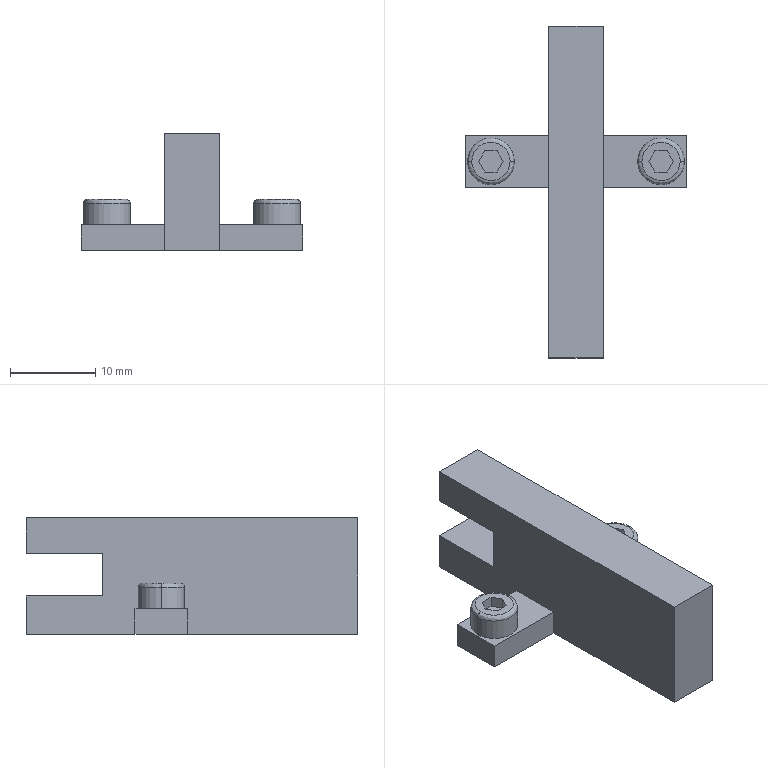Part | SolidWorks | features BaseBody 1 | 1 solid | 48 faces | box 26 x 39 x 13.7 mm | volume 3551 mm3 | plane 36 | cylinder 8 | spline 4 | commonest cylinder face diameters 3.2 x4 5.5 x4
STEP:
#1=CARTESIAN_POINT('',(-7.75,0.,6.));
#2=VERTEX_POINT('',#1);
#3=CARTESIAN_POINT('',(-12.25,0.,6.));
#4=VERTEX_POINT('',#3);
#5=CARTESIAN_POINT('',(-7.75,0.,6.));
#6=CARTESIAN_POINT('',(-7.75,-4.5,6.));
#7=CARTESIAN_POINT('',(-12.25,-4.5,6.));
#8=CARTESIAN_POINT('',(-12.25,0.,6.));
#9=(BOUNDED_CURVE()B_SPLINE_CURVE(3,(#5,#6,#7,#8),.UNSPECIFIED.,.F.,.F.)B_SPLINE_CURVE_WITH_KNOTS((4,4),(0.,1.),.UNSPECIFIED.)CURVE()GEOMETRIC_REPRESENTATION_ITEM()RATIONAL_B_SPLINE_CURVE((1.,0.3333,0.3333,1.))REPRESENTATION_ITEM(''));
#10=EDGE_CURVE('',#2,#4,#9,.T.);
#11=ORIENTED_EDGE('',*,*,#10,.T.);
#12=CARTESIAN_POINT('',(-12.75,0.,5.5));
#13=VERTEX_POINT('',#12);
#14=CARTESIAN_POINT('',(-12.25,0.,5.5));
#15=DIRECTION('',(0.,-1.,0.));
#16=DIRECTION('',(-1.,0.,0.));
#17=AXIS2_PLACEMENT_3D('',#14,#15,#16);
#18=CIRCLE('',#17,0.5);
#19=EDGE_CURVE('',#4,#13,#18,.T.);
#20=ORIENTED_EDGE('',*,*,#19,.T.);
#21=CARTESIAN_POINT('',(-7.25,0.,5.5));
#22=VERTEX_POINT('',#21);
#23=CARTESIAN_POINT('',(-10.,0.,5.5));
#24=DIRECTION('',(0.,0.,-1.));
#25=DIRECTION('',(-1.,0.,0.));
#26=AXIS2_PLACEMENT_3D('',#23,#24,#25);
#27=CIRCLE('',#26,2.75);
#28=EDGE_CURVE('',#22,#13,#27,.T.);
#29=ORIENTED_EDGE('',*,*,#28,.F.);
#30=CARTESIAN_POINT('',(-7.75,0.,5.5));
#31=DIRECTION('',(0.,1.,0.));
#32=DIRECTION('',(1.,0.,0.));
#33=AXIS2_PLACEMENT_3D('',#30,#31,#32);
#34=CIRCLE('',#33,0.5);
#35=EDGE_CURVE('',#2,#22,#34,.T.);
#36=ORIENTED_EDGE('',*,*,#35,.F.);
#37=EDGE_LOOP('',(#11,#20,#29,#36));
#38=FACE_OUTER_BOUND('',#37,.T.);
#39=CARTESIAN_POINT('',(-12.25,0.,6.));
#40=CARTESIAN_POINT('',(-12.25,-4.5,6.));
#41=CARTESIAN_POINT('',(-7.75,-4.5,6.));
#42=CARTESIAN_POINT('',(-7.75,0.,6.));
#43=CARTESIAN_POINT('',(-12.543,0.,6.));
#44=CARTESIAN_POINT('',(-12.543,-5.086,6.));
#45=CARTESIAN_POINT('',(-7.457,-5.086,6.));
#46=CARTESIAN_POINT('',(-7.457,0.,6.));
#47=CARTESIAN_POINT('',(-12.75,0.,5.793));
#48=CARTESIAN_POINT('',(-12.75,-5.5,5.793));
#49=CARTESIAN_POINT('',(-7.25,-5.5,5.793));
#50=CARTESIAN_POINT('',(-7.25,0.,5.793));
#51=CARTESIAN_POINT('',(-12.75,0.,5.5));
#52=CARTESIAN_POINT('',(-12.75,-5.5,5.5));
#53=CARTESIAN_POINT('',(-7.25,-5.5,5.5));
#54=CARTESIAN_POINT('',(-7.25,0.,5.5));
#55=(BOUNDED_SURFACE()B_SPLINE_SURFACE(3,3,((#39,#40,#41,#42),(#43,#44,#45,#46),(#47,#48,#49,#50),(#51,#52,#53,#54)),.UNSPECIFIED.,.F.,.F.,.F.)B_SPLINE_SURFACE_WITH_KNOTS((4,4),(4,4),(0.,1.),(0.,1.),.UNSPECIFIED.)GEOMETRIC_REPRESENTATION_ITEM()RATIONAL_B_SPLINE_SURFACE(((1.,0.3333,0.3333,1.),(0.8047,0.2682,0.2682,0.8047),(0.8047,0.2682,0.2682,0.8047),(1.,0.3333,0.3333,1.)))REPRESENTATION_ITEM('')SURFACE());
#56=ADVANCED_FACE('',(#38),#55,.T.);
#57=CARTESIAN_POINT('',(12.25,0.,6.));
#58=VERTEX_POINT('',#57);
#59=CARTESIAN_POINT('',(7.75,0.,6.));
#60=VERTEX_POINT('',#59);
#61=CARTESIAN_POINT('',(12.25,0.,6.));
#62=CARTESIAN_POINT('',(12.25,-4.5,6.));
#63=CARTESIAN_POINT('',(7.75,-4.5,6.));
#64=CARTESIAN_POINT('',(7.75,0.,6.));
#65=(BOUNDED_CURVE()B_SPLINE_CURVE(3,(#61,#62,#63,#64),.UNSPECIFIED.,.F.,.F.)B_SPLINE_CURVE_WITH_KNOTS((4,4),(0.,1.),.UNSPECIFIED.)CURVE()GEOMETRIC_REPRESENTATION_ITEM()RATIONAL_B_SPLINE_CURVE((1.,0.3333,0.3333,1.))REPRESENTATION_ITEM(''));
#66=EDGE_CURVE('',#58,#60,#65,.T.);
#67=ORIENTED_EDGE('',*,*,#66,.T.);
#68=CARTESIAN_POINT('',(7.25,0.,5.5));
#69=VERTEX_POINT('',#68);
#70=CARTESIAN_POINT('',(7.75,0.,5.5));
#71=DIRECTION('',(0.,-1.,0.));
#72=DIRECTION('',(-1.,0.,0.));
#73=AXIS2_PLACEMENT_3D('',#70,#71,#72);
#74=CIRCLE('',#73,0.5);
#75=EDGE_CURVE('',#60,#69,#74,.T.);
#76=ORIENTED_EDGE('',*,*,#75,.T.);
#77=CARTESIAN_POINT('',(12.75,0.,5.5));
#78=VERTEX_POINT('',#77);
#79=CARTESIAN_POINT('',(10.,0.,5.5));
#80=DIRECTION('',(0.,0.,-1.));
#81=DIRECTION('',(-1.,0.,0.));
#82=AXIS2_PLACEMENT_3D('',#79,#80,#81);
#83=CIRCLE('',#82,2.75);
#84=EDGE_CURVE('',#78,#69,#83,.T.);
#85=ORIENTED_EDGE('',*,*,#84,.F.);
#86=CARTESIAN_POINT('',(12.25,0.,5.5));
#87=DIRECTION('',(0.,1.,0.));
#88=DIRECTION('',(1.,0.,0.));
#89=AXIS2_PLACEMENT_3D('',#86,#87,#88);
#90=CIRCLE('',#89,0.5);
#91=EDGE_CURVE('',#58,#78,#90,.T.);
#92=ORIENTED_EDGE('',*,*,#91,.F.);
#93=EDGE_LOOP('',(#67,#76,#85,#92));
#94=FACE_OUTER_BOUND('',#93,.T.);
#95=CARTESIAN_POINT('',(7.75,0.,6.));
#96=CARTESIAN_POINT('',(7.75,-4.5,6.));
#97=CARTESIAN_POINT('',(12.25,-4.5,6.));
#98=CARTESIAN_POINT('',(12.25,0.,6.));
#99=CARTESIAN_POINT('',(7.457,0.,6.));
#100=CARTESIAN_POINT('',(7.457,-5.086,6.));
#101=CARTESIAN_POINT('',(12.543,-5.086,6.));
#102=CARTESIAN_POINT('',(12.543,0.,6.));
#103=CARTESIAN_POINT('',(7.25,0.,5.793));
#104=CARTESIAN_POINT('',(7.25,-5.5,5.793));
#105=CARTESIAN_POINT('',(12.75,-5.5,5.793));
#106=CARTESIAN_POINT('',(12.75,0.,5.793));
#107=CARTESIAN_POINT('',(7.25,0.,5.5));
#108=CARTESIAN_POINT('',(7.25,-5.5,5.5));
#109=CARTESIAN_POINT('',(12.75,-5.5,5.5));
#110=CARTESIAN_POINT('',(12.75,0.,5.5));
#111=(BOUNDED_SURFACE()B_SPLINE_SURFACE(3,3,((#95,#96,#97,#98),(#99,#100,#101,#102),(#103,#104,#105,#106),(#107,#108,#109,#110)),.UNSPECIFIED.,.F.,.F.,.F.)B_SPLINE_SURFACE_WITH_KNOTS((4,4),(4,4),(0.,1.),(0.,1.),.UNSPECIFIED.)GEOMETRIC_REPRESENTATION_ITEM()RATIONAL_B_SPLINE_SURFACE(((1.,0.3333,0.3333,1.),(0.8047,0.2682,0.2682,0.8047),(0.8047,0.2682,0.2682,0.8047),(1.,0.3333,0.3333,1.)))REPRESENTATION_ITEM('')SURFACE());
#112=ADVANCED_FACE('',(#94),#111,.T.);
#113=CARTESIAN_POINT('',(-8.4,0.,0.));
#114=VERTEX_POINT('',#113);
#115=CARTESIAN_POINT('',(-11.6,0.,0.));
#116=VERTEX_POINT('',#115);
#117=CARTESIAN_POINT('',(-10.,0.,0.));
#118=DIRECTION('',(0.,0.,-1.));
#119=DIRECTION('',(1.,0.,0.));
#120=AXIS2_PLACEMENT_3D('',#117,#118,#119);
#121=CIRCLE('',#120,1.6);
#122=EDGE_CURVE('',#114,#116,#121,.T.);
#123=ORIENTED_EDGE('',*,*,#122,.T.);
#124=CARTESIAN_POINT('',(-11.6,0.,3.));
#125=VERTEX_POINT('',#124);
#126=CARTESIAN_POINT('',(-11.6,0.,1.5));
#127=DIRECTION('',(0.,0.,1.));
#128=VECTOR('',#127,1000.);
#129=LINE('',#126,#128);
#130=EDGE_CURVE('',#116,#125,#129,.T.);
#131=ORIENTED_EDGE('',*,*,#130,.T.);
#132=CARTESIAN_POINT('',(-8.4,0.,3.));
#133=VERTEX_POINT('',#132);
#134=CARTESIAN_POINT('',(-10.,0.,3.));
#135=DIRECTION('',(0.,0.,-1.));
#136=DIRECTION('',(1.,0.,0.));
#137=AXIS2_PLACEMENT_3D('',#134,#135,#136);
#138=CIRCLE('',#137,1.6);
#139=EDGE_CURVE('',#133,#125,#138,.T.);
#140=ORIENTED_EDGE('',*,*,#139,.F.);
#141=CARTESIAN_POINT('',(-8.4,0.,1.5));
#142=DIRECTION('',(0.,0.,1.));
#143=VECTOR('',#142,1000.);
#144=LINE('',#141,#143);
#145=EDGE_CURVE('',#114,#133,#144,.T.);
#146=ORIENTED_EDGE('',*,*,#145,.F.);
#147=EDGE_LOOP('',(#123,#131,#140,#146));
#148=FACE_OUTER_BOUND('',#147,.T.);
#149=CARTESIAN_POINT('',(-10.,0.,1.5));
#150=DIRECTION('',(0.,0.,1.));
#151=DIRECTION('',(1.,0.,0.));
#152=AXIS2_PLACEMENT_3D('',#149,#150,#151);
#153=CYLINDRICAL_SURFACE('',#152,1.6);
#154=ADVANCED_FACE('',(#148),#153,.F.);
#155=CARTESIAN_POINT('',(11.6,0.,3.));
#156=VERTEX_POINT('',#155);
#157=CARTESIAN_POINT('',(8.4,0.,3.));
#158=VERTEX_POINT('',#157);
#159=CARTESIAN_POINT('',(10.,0.,3.));
#160=DIRECTION('',(0.,0.,-1.));
#161=DIRECTION('',(-1.,0.,0.));
#162=AXIS2_PLACEMENT_3D('',#159,#160,#161);
#163=CIRCLE('',#162,1.6);
#164=EDGE_CURVE('',#156,#158,#163,.T.);
#165=ORIENTED_EDGE('',*,*,#164,.F.);
#166=CARTESIAN_POINT('',(11.6,0.,0.));
#167=VERTEX_POINT('',#166);
#168=CARTESIAN_POINT('',(11.6,0.,3.));
#169=DIRECTION('',(0.,0.,-1.));
#170=VECTOR('',#169,1000.);
#171=LINE('',#168,#170);
#172=EDGE_CURVE('',#156,#167,#171,.T.);
#173=ORIENTED_EDGE('',*,*,#172,.T.);
#174=CARTESIAN_POINT('',(8.4,0.,0.));
#175=VERTEX_POINT('',#174);
#176=CARTESIAN_POINT('',(10.,0.,0.));
#177=DIRECTION('',(0.,0.,-1.));
#178=DIRECTION('',(-1.,0.,0.));
#179=AXIS2_PLACEMENT_3D('',#176,#177,#178);
#180=CIRCLE('',#179,1.6);
#181=EDGE_CURVE('',#167,#175,#180,.T.);
#182=ORIENTED_EDGE('',*,*,#181,.T.);
#183=CARTESIAN_POINT('',(8.4,0.,3.));
#184=DIRECTION('',(0.,0.,-1.));
#185=VECTOR('',#184,1000.);
#186=LINE('',#183,#185);
#187=EDGE_CURVE('',#158,#175,#186,.T.);
#188=ORIENTED_EDGE('',*,*,#187,.F.);
#189=EDGE_LOOP('',(#165,#173,#182,#188));
#190=FACE_OUTER_BOUND('',#189,.T.);
#191=CARTESIAN_POINT('',(10.,0.,3.));
#192=DIRECTION('',(0.,0.,-1.));
#193=DIRECTION('',(-1.,0.,0.));
#194=AXIS2_PLACEMENT_3D('',#191,#192,#193);
#195=CYLINDRICAL_SURFACE('',#194,1.6);
#196=ADVANCED_FACE('',(#190),#195,.F.);
#197=CARTESIAN_POINT('',(-10.,0.,5.5));
#198=DIRECTION('',(0.,0.,-1.));
#199=DIRECTION('',(-1.,0.,0.));
#200=AXIS2_PLACEMENT_3D('',#197,#198,#199);
#201=CIRCLE('',#200,2.75);
#202=EDGE_CURVE('',#13,#22,#201,.T.);
#203=ORIENTED_EDGE('',*,*,#202,.T.);
#204=CARTESIAN_POINT('',(-7.25,0.,3.));
#205=VERTEX_POINT('',#204);
#206=CARTESIAN_POINT('',(-7.25,0.,6.));
#207=DIRECTION('',(0.,0.,-1.));
#208=VECTOR('',#207,1000.);
#209=LINE('',#206,#208);
#210=EDGE_CURVE('',#22,#205,#209,.T.);
#211=ORIENTED_EDGE('',*,*,#210,.T.);
#212=CARTESIAN_POINT('',(-12.75,0.,3.));
#213=VERTEX_POINT('',#212);
#214=CARTESIAN_POINT('',(-10.,0.,3.));
#215=DIRECTION('',(0.,0.,-1.));
#216=DIRECTION('',(-1.,0.,0.));
#217=AXIS2_PLACEMENT_3D('',#214,#215,#216);
#218=CIRCLE('',#217,2.75);
#219=EDGE_CURVE('',#213,#205,#218,.T.);
#220=ORIENTED_EDGE('',*,*,#219,.F.);
#221=CARTESIAN_POINT('',(-12.75,0.,6.));
#222=DIRECTION('',(0.,0.,-1.));
#223=VECTOR('',#222,1000.);
#224=LINE('',#221,#223);
#225=EDGE_CURVE('',#13,#213,#224,.T.);
#226=ORIENTED_EDGE('',*,*,#225,.F.);
#227=EDGE_LOOP('',(#203,#211,#220,#226));
#228=FACE_OUTER_BOUND('',#227,.T.);
#229=CARTESIAN_POINT('',(-10.,0.,6.));
#230=DIRECTION('',(0.,0.,-1.));
#231=DIRECTION('',(-1.,0.,0.));
#232=AXIS2_PLACEMENT_3D('',#229,#230,#231);
#233=CYLINDRICAL_SURFACE('',#232,2.75);
#234=ADVANCED_FACE('',(#228),#233,.T.);
#235=CARTESIAN_POINT('',(10.,0.,5.5));
#236=DIRECTION('',(0.,0.,-1.));
#237=DIRECTION('',(-1.,0.,0.));
#238=AXIS2_PLACEMENT_3D('',#235,#236,#237);
#239=CIRCLE('',#238,2.75);
#240=EDGE_CURVE('',#69,#78,#239,.T.);
#241=ORIENTED_EDGE('',*,*,#240,.T.);
#242=CARTESIAN_POINT('',(12.75,0.,3.));
#243=VERTEX_POINT('',#242);
#244=CARTESIAN_POINT('',(12.75,0.,6.));
#245=DIRECTION('',(0.,0.,-1.));
#246=VECTOR('',#245,1000.);
#247=LINE('',#244,#246);
#248=EDGE_CURVE('',#78,#243,#247,.T.);
#249=ORIENTED_EDGE('',*,*,#248,.T.);
#250=CARTESIAN_POINT('',(7.25,0.,3.));
#251=VERTEX_POINT('',#250);
#252=CARTESIAN_POINT('',(10.,0.,3.));
#253=DIRECTION('',(0.,0.,-1.));
#254=DIRECTION('',(-1.,0.,0.));
#255=AXIS2_PLACEMENT_3D('',#252,#253,#254);
#256=CIRCLE('',#255,2.75);
#257=EDGE_CURVE('',#251,#243,#256,.T.);
#258=ORIENTED_EDGE('',*,*,#257,.F.);
#259=CARTESIAN_POINT('',(7.25,0.,6.));
#260=DIRECTION('',(0.,0.,-1.));
#261=VECTOR('',#260,1000.);
#262=LINE('',#259,#261);
#263=EDGE_CURVE('',#69,#251,#262,.T.);
#264=ORIENTED_EDGE('',*,*,#263,.F.);
#265=EDGE_LOOP('',(#241,#249,#258,#264));
#266=FACE_OUTER_BOUND('',#265,.T.);
#267=CARTESIAN_POINT('',(10.,0.,6.));
#268=DIRECTION('',(0.,0.,-1.));
#269=DIRECTION('',(-1.,0.,0.));
#270=AXIS2_PLACEMENT_3D('',#267,#268,#269);
#271=CYLINDRICAL_SURFACE('',#270,2.75);
#272=ADVANCED_FACE('',(#266),#271,.T.);
#273=CARTESIAN_POINT('',(-3.175,-23.1,13.7));
#274=VERTEX_POINT('',#273);
#275=CARTESIAN_POINT('',(-3.175,15.9,13.7));
#276=VERTEX_POINT('',#275);
#277=CARTESIAN_POINT('',(-3.175,-23.1,13.7));
#278=DIRECTION('',(0.,1.,0.));
#279=VECTOR('',#278,1000.);
#280=LINE('',#277,#279);
#281=EDGE_CURVE('',#274,#276,#280,.T.);
#282=ORIENTED_EDGE('',*,*,#281,.T.);
#283=CARTESIAN_POINT('',(-3.175,15.9,9.5));
#284=VERTEX_POINT('',#283);
#285=CARTESIAN_POINT('',(-3.175,15.9,0.));
#286=DIRECTION('',(0.,0.,-1.));
#287=VECTOR('',#286,1000.);
#288=LINE('',#285,#287);
#289=EDGE_CURVE('',#276,#284,#288,.T.);
#290=ORIENTED_EDGE('',*,*,#289,.T.);
#291=CARTESIAN_POINT('',(-3.175,6.9,9.5));
#292=VERTEX_POINT('',#291);
#293=CARTESIAN_POINT('',(-3.175,-23.1,9.5));
#294=DIRECTION('',(0.,-1.,0.));
#295=VECTOR('',#294,1000.);
#296=LINE('',#293,#295);
#297=EDGE_CURVE('',#284,#292,#296,.T.);
#298=ORIENTED_EDGE('',*,*,#297,.T.);
#299=CARTESIAN_POINT('',(-3.175,6.9,4.5));
#300=VERTEX_POINT('',#299);
#301=CARTESIAN_POINT('',(-3.175,6.9,0.));
#302=DIRECTION('',(0.,0.,-1.));
#303=VECTOR('',#302,1000.);
#304=LINE('',#301,#303);
#305=EDGE_CURVE('',#292,#300,#304,.T.);
#306=ORIENTED_EDGE('',*,*,#305,.T.);
#307=CARTESIAN_POINT('',(-3.175,15.9,4.5));
#308=VERTEX_POINT('',#307);
#309=CARTESIAN_POINT('',(-3.175,-23.1,4.5));
#310=DIRECTION('',(0.,1.,0.));
#311=VECTOR('',#310,1000.);
#312=LINE('',#309,#311);
#313=EDGE_CURVE('',#300,#308,#312,.T.);
#314=ORIENTED_EDGE('',*,*,#313,.T.);
#315=CARTESIAN_POINT('',(-3.175,15.9,0.));
#316=VERTEX_POINT('',#315);
#317=CARTESIAN_POINT('',(-3.175,15.9,0.));
#318=DIRECTION('',(0.,0.,-1.));
#319=VECTOR('',#318,1000.);
#320=LINE('',#317,#319);
#321=EDGE_CURVE('',#308,#316,#320,.T.);
#322=ORIENTED_EDGE('',*,*,#321,.T.);
#323=CARTESIAN_POINT('',(-3.175,3.1,0.));
#324=VERTEX_POINT('',#323);
#325=CARTESIAN_POINT('',(-3.175,-23.1,0.));
#326=DIRECTION('',(0.,-1.,0.));
#327=VECTOR('',#326,1000.);
#328=LINE('',#325,#327);
#329=EDGE_CURVE('',#316,#324,#328,.T.);
#330=ORIENTED_EDGE('',*,*,#329,.T.);
#331=CARTESIAN_POINT('',(-3.175,3.1,3.));
#332=VERTEX_POINT('',#331);
#333=CARTESIAN_POINT('',(-3.175,3.1,0.));
#334=DIRECTION('',(0.,0.,1.));
#335=VECTOR('',#334,1000.);
#336=LINE('',#333,#335);
#337=EDGE_CURVE('',#324,#332,#336,.T.);
#338=ORIENTED_EDGE('',*,*,#337,.T.);
#339=CARTESIAN_POINT('',(-3.175,-3.1,3.));
#340=VERTEX_POINT('',#339);
#341=CARTESIAN_POINT('',(-3.175,-23.1,3.));
#342=DIRECTION('',(0.,-1.,0.));
#343=VECTOR('',#342,1000.);
#344=LINE('',#341,#343);
#345=EDGE_CURVE('',#332,#340,#344,.T.);
#346=ORIENTED_EDGE('',*,*,#345,.T.);
#347=CARTESIAN_POINT('',(-3.175,-3.1,0.));
#348=VERTEX_POINT('',#347);
#349=CARTESIAN_POINT('',(-3.175,-3.1,0.));
#350=DIRECTION('',(0.,0.,-1.));
#351=VECTOR('',#350,1000.);
#352=LINE('',#349,#351);
#353=EDGE_CURVE('',#340,#348,#352,.T.);
#354=ORIENTED_EDGE('',*,*,#353,.T.);
#355=CARTESIAN_POINT('',(-3.175,-23.1,0.));
#356=VERTEX_POINT('',#355);
#357=CARTESIAN_POINT('',(-3.175,-23.1,0.));
#358=DIRECTION('',(0.,-1.,0.));
#359=VECTOR('',#358,1000.);
#360=LINE('',#357,#359);
#361=EDGE_CURVE('',#348,#356,#360,.T.);
#362=ORIENTED_EDGE('',*,*,#361,.T.);
#363=CARTESIAN_POINT('',(-3.175,-23.1,0.));
#364=DIRECTION('',(0.,0.,1.));
#365=VECTOR('',#364,1000.);
#366=LINE('',#363,#365);
#367=EDGE_CURVE('',#356,#274,#366,.T.);
#368=ORIENTED_EDGE('',*,*,#367,.T.);
#369=EDGE_LOOP('',(#282,#290,#298,#306,#314,#322,#330,#338,#346,#354,#362,#368));
#370=FACE_OUTER_BOUND('',#369,.T.);
#371=CARTESIAN_POINT('',(-3.175,-23.1,0.));
#372=DIRECTION('',(-1.,0.,0.));
#373=DIRECTION('',(0.,0.,1.));
#374=AXIS2_PLACEMENT_3D('',#371,#372,#373);
#375=PLANE('',#374);
#376=ADVANCED_FACE('',(#370),#375,.T.);
#377=CARTESIAN_POINT('',(3.175,15.9,9.5));
#378=VERTEX_POINT('',#377);
#379=CARTESIAN_POINT('',(-3.175,15.9,9.5));
#380=DIRECTION('',(-1.,0.,0.));
#381=VECTOR('',#380,1000.);
#382=LINE('',#379,#381);
#383=EDGE_CURVE('',#378,#284,#382,.T.);
#384=ORIENTED_EDGE('',*,*,#383,.T.);
#385=ORIENTED_EDGE('',*,*,#289,.F.);
#386=CARTESIAN_POINT('',(3.175,15.9,13.7));
#387=VERTEX_POINT('',#386);
#388=CARTESIAN_POINT('',(-3.175,15.9,13.7));
#389=DIRECTION('',(1.,0.,0.));
#390=VECTOR('',#389,1000.);
#391=LINE('',#388,#390);
#392=EDGE_CURVE('',#276,#387,#391,.T.);
#393=ORIENTED_EDGE('',*,*,#392,.T.);
#394=CARTESIAN_POINT('',(3.175,15.9,0.));
#395=DIRECTION('',(0.,0.,-1.));
#396=VECTOR('',#395,1000.);
#397=LINE('',#394,#396);
#398=EDGE_CURVE('',#387,#378,#397,.T.);
#399=ORIENTED_EDGE('',*,*,#398,.T.);
#400=EDGE_LOOP('',(#384,#385,#393,#399));
#401=FACE_OUTER_BOUND('',#400,.T.);
#402=CARTESIAN_POINT('',(-3.175,15.9,0.));
#403=DIRECTION('',(0.,1.,0.));
#404=DIRECTION('',(0.,0.,1.));
#405=AXIS2_PLACEMENT_3D('',#402,#403,#404);
#406=PLANE('',#405);
#407=ADVANCED_FACE('',(#401),#406,.T.);
#408=ORIENTED_EDGE('',*,*,#281,.F.);
#409=CARTESIAN_POINT('',(3.175,-23.1,13.7));
#410=VERTEX_POINT('',#409);
#411=CARTESIAN_POINT('',(0.,-23.1,13.7));
#412=DIRECTION('',(1.,0.,0.));
#413=VECTOR('',#412,1000.);
#414=LINE('',#411,#413);
#415=EDGE_CURVE('',#274,#410,#414,.T.);
#416=ORIENTED_EDGE('',*,*,#415,.T.);
#417=CARTESIAN_POINT('',(3.175,-3.6,13.7));
#418=DIRECTION('',(0.,1.,0.));
#419=VECTOR('',#418,1000.);
#420=LINE('',#417,#419);
#421=EDGE_CURVE('',#410,#387,#420,.T.);
#422=ORIENTED_EDGE('',*,*,#421,.T.);
#423=ORIENTED_EDGE('',*,*,#392,.F.);
#424=EDGE_LOOP('',(#408,#416,#422,#423));
#425=FACE_OUTER_BOUND('',#424,.T.);
#426=CARTESIAN_POINT('',(0.,-3.6,13.7));
#427=DIRECTION('',(0.,0.,1.));
#428=DIRECTION('',(1.,0.,0.));
#429=AXIS2_PLACEMENT_3D('',#426,#427,#428);
#430=PLANE('',#429);
#431=ADVANCED_FACE('',(#425),#430,.T.);
#432=ORIENTED_EDGE('',*,*,#415,.F.);
#433=ORIENTED_EDGE('',*,*,#367,.F.);
#434=CARTESIAN_POINT('',(3.175,-23.1,0.));
#435=VERTEX_POINT('',#434);
#436=CARTESIAN_POINT('',(3.175,-23.1,0.));
#437=DIRECTION('',(1.,0.,0.));
#438=VECTOR('',#437,1000.);
#439=LINE('',#436,#438);
#440=EDGE_CURVE('',#356,#435,#439,.T.);
#441=ORIENTED_EDGE('',*,*,#440,.T.);
#442=CARTESIAN_POINT('',(3.175,-23.1,0.));
#443=DIRECTION('',(0.,0.,1.));
#444=VECTOR('',#443,1000.);
#445=LINE('',#442,#444);
#446=EDGE_CURVE('',#435,#410,#445,.T.);
#447=ORIENTED_EDGE('',*,*,#446,.T.);
#448=EDGE_LOOP('',(#432,#433,#441,#447));
#449=FACE_OUTER_BOUND('',#448,.T.);
#450=CARTESIAN_POINT('',(3.175,-23.1,0.));
#451=DIRECTION('',(0.,-1.,0.));
#452=DIRECTION('',(0.,0.,-1.));
#453=AXIS2_PLACEMENT_3D('',#450,#451,#452);
#454=PLANE('',#453);
#455=ADVANCED_FACE('',(#449),#454,.T.);
#456=CARTESIAN_POINT('',(-13.,3.1,0.));
#457=VERTEX_POINT('',#456);
#458=CARTESIAN_POINT('',(0.,3.1,0.));
#459=DIRECTION('',(-1.,0.,0.));
#460=VECTOR('',#459,1000.);
#461=LINE('',#458,#460);
#462=EDGE_CURVE('',#324,#457,#461,.T.);
#463=ORIENTED_EDGE('',*,*,#462,.F.);
#464=ORIENTED_EDGE('',*,*,#329,.F.);
#465=CARTESIAN_POINT('',(3.175,15.9,0.));
#466=VERTEX_POINT('',#465);
#467=CARTESIAN_POINT('',(0.,15.9,0.));
#468=DIRECTION('',(-1.,0.,0.));
#469=VECTOR('',#468,1000.);
#470=LINE('',#467,#469);
#471=EDGE_CURVE('',#466,#316,#470,.T.);
#472=ORIENTED_EDGE('',*,*,#471,.F.);
#473=CARTESIAN_POINT('',(3.175,3.1,0.));
#474=VERTEX_POINT('',#473);
#475=CARTESIAN_POINT('',(3.175,0.,0.));
#476=DIRECTION('',(0.,1.,0.));
#477=VECTOR('',#476,1000.);
#478=LINE('',#475,#477);
#479=EDGE_CURVE('',#474,#466,#478,.T.);
#480=ORIENTED_EDGE('',*,*,#479,.F.);
#481=CARTESIAN_POINT('',(13.,3.1,0.));
#482=VERTEX_POINT('',#481);
#483=CARTESIAN_POINT('',(0.,3.1,0.));
#484=DIRECTION('',(-1.,0.,0.));
#485=VECTOR('',#484,1000.);
#486=LINE('',#483,#485);
#487=EDGE_CURVE('',#482,#474,#486,.T.);
#488=ORIENTED_EDGE('',*,*,#487,.F.);
#489=CARTESIAN_POINT('',(13.,-3.1,0.));
#490=VERTEX_POINT('',#489);
#491=CARTESIAN_POINT('',(13.,0.,0.));
#492=DIRECTION('',(0.,1.,0.));
#493=VECTOR('',#492,1000.);
#494=LINE('',#491,#493);
#495=EDGE_CURVE('',#490,#482,#494,.T.);
#496=ORIENTED_EDGE('',*,*,#495,.F.);
#497=CARTESIAN_POINT('',(3.175,-3.1,0.));
#498=VERTEX_POINT('',#497);
#499=CARTESIAN_POINT('',(0.,-3.1,0.));
#500=DIRECTION('',(1.,0.,0.));
#501=VECTOR('',#500,1000.);
#502=LINE('',#499,#501);
#503=EDGE_CURVE('',#498,#490,#502,.T.);
#504=ORIENTED_EDGE('',*,*,#503,.F.);
#505=CARTESIAN_POINT('',(3.175,0.,0.));
#506=DIRECTION('',(0.,1.,0.));
#507=VECTOR('',#506,1000.);
#508=LINE('',#505,#507);
#509=EDGE_CURVE('',#435,#498,#508,.T.);
#510=ORIENTED_EDGE('',*,*,#509,.F.);
#511=ORIENTED_EDGE('',*,*,#440,.F.);
#512=ORIENTED_EDGE('',*,*,#361,.F.);
#513=CARTESIAN_POINT('',(-13.,-3.1,0.));
#514=VERTEX_POINT('',#513);
#515=CARTESIAN_POINT('',(0.,-3.1,0.));
#516=DIRECTION('',(1.,0.,0.));
#517=VECTOR('',#516,1000.);
#518=LINE('',#515,#517);
#519=EDGE_CURVE('',#514,#348,#518,.T.);
#520=ORIENTED_EDGE('',*,*,#519,.F.);
#521=CARTESIAN_POINT('',(-13.,0.,0.));
#522=DIRECTION('',(0.,-1.,0.));
#523=VECTOR('',#522,1000.);
#524=LINE('',#521,#523);
#525=EDGE_CURVE('',#457,#514,#524,.T.);
#526=ORIENTED_EDGE('',*,*,#525,.F.);
#527=EDGE_LOOP('',(#463,#464,#472,#480,#488,#496,#504,#510,#511,#512,#520,#526));
#528=FACE_OUTER_BOUND('',#527,.T.);
#529=ORIENTED_EDGE('',*,*,#122,.F.);
#530=CARTESIAN_POINT('',(-10.,0.,0.));
#531=DIRECTION('',(0.,0.,-1.));
#532=DIRECTION('',(1.,0.,0.));
#533=AXIS2_PLACEMENT_3D('',#530,#531,#532);
#534=CIRCLE('',#533,1.6);
#535=EDGE_CURVE('',#116,#114,#534,.T.);
#536=ORIENTED_EDGE('',*,*,#535,.F.);
#537=EDGE_LOOP('',(#529,#536));
#538=FACE_BOUND('',#537,.T.);
#539=CARTESIAN_POINT('',(10.,0.,0.));
#540=DIRECTION('',(0.,0.,-1.));
#541=DIRECTION('',(-1.,0.,0.));
#542=AXIS2_PLACEMENT_3D('',#539,#540,#541);
#543=CIRCLE('',#542,1.6);
#544=EDGE_CURVE('',#175,#167,#543,.T.);
#545=ORIENTED_EDGE('',*,*,#544,.F.);
#546=ORIENTED_EDGE('',*,*,#181,.F.);
#547=EDGE_LOOP('',(#545,#546));
#548=FACE_BOUND('',#547,.T.);
#549=CARTESIAN_POINT('',(0.,0.,0.));
#550=DIRECTION('',(0.,0.,1.));
#551=DIRECTION('',(1.,0.,0.));
#552=AXIS2_PLACEMENT_3D('',#549,#550,#551);
#553=PLANE('',#552);
#554=ADVANCED_FACE('',(#528,#538,#548),#553,.F.);
#555=ORIENTED_EDGE('',*,*,#353,.F.);
#556=CARTESIAN_POINT('',(-13.,-3.1,3.));
#557=VERTEX_POINT('',#556);
#558=CARTESIAN_POINT('',(13.,-3.1,3.));
#559=DIRECTION('',(-1.,0.,0.));
#560=VECTOR('',#559,1000.);
#561=LINE('',#558,#560);
#562=EDGE_CURVE('',#340,#557,#561,.T.);
#563=ORIENTED_EDGE('',*,*,#562,.T.);
#564=CARTESIAN_POINT('',(-13.,-3.1,0.));
#565=DIRECTION('',(0.,0.,-1.));
#566=VECTOR('',#565,1000.);
#567=LINE('',#564,#566);
#568=EDGE_CURVE('',#557,#514,#567,.T.);
#569=ORIENTED_EDGE('',*,*,#568,.T.);
#570=ORIENTED_EDGE('',*,*,#519,.T.);
#571=EDGE_LOOP('',(#555,#563,#569,#570));
#572=FACE_OUTER_BOUND('',#571,.T.);
#573=CARTESIAN_POINT('',(13.,-3.1,0.));
#574=DIRECTION('',(0.,-1.,0.));
#575=DIRECTION('',(0.,0.,-1.));
#576=AXIS2_PLACEMENT_3D('',#573,#574,#575);
#577=PLANE('',#576);
#578=ADVANCED_FACE('',(#572),#577,.T.);
#579=ORIENTED_EDGE('',*,*,#219,.T.);
#580=CARTESIAN_POINT('',(-10.,0.,3.));
#581=DIRECTION('',(0.,0.,-1.));
#582=DIRECTION('',(-1.,0.,0.));
#583=AXIS2_PLACEMENT_3D('',#580,#581,#582);
#584=CIRCLE('',#583,2.75);
#585=EDGE_CURVE('',#205,#213,#584,.T.);
#586=ORIENTED_EDGE('',*,*,#585,.T.);
#587=EDGE_LOOP('',(#579,#586));
#588=FACE_BOUND('',#587,.T.);
#589=ORIENTED_EDGE('',*,*,#345,.F.);
#590=CARTESIAN_POINT('',(-13.,3.1,3.));
#591=VERTEX_POINT('',#590);
#592=CARTESIAN_POINT('',(0.,3.1,3.));
#593=DIRECTION('',(-1.,0.,0.));
#594=VECTOR('',#593,1000.);
#595=LINE('',#592,#594);
#596=EDGE_CURVE('',#332,#591,#595,.T.);
#597=ORIENTED_EDGE('',*,*,#596,.T.);
#598=CARTESIAN_POINT('',(-13.,0.,3.));
#599=DIRECTION('',(0.,-1.,0.));
#600=VECTOR('',#599,1000.);
#601=LINE('',#598,#600);
#602=EDGE_CURVE('',#591,#557,#601,.T.);
#603=ORIENTED_EDGE('',*,*,#602,.T.);
#604=ORIENTED_EDGE('',*,*,#562,.F.);
#605=EDGE_LOOP('',(#589,#597,#603,#604));
#606=FACE_OUTER_BOUND('',#605,.T.);
#607=CARTESIAN_POINT('',(0.,0.,3.));
#608=DIRECTION('',(0.,0.,1.));
#609=DIRECTION('',(1.,0.,0.));
#610=AXIS2_PLACEMENT_3D('',#607,#608,#609);
#611=PLANE('',#610);
#612=ADVANCED_FACE('',(#588,#606),#611,.T.);
#613=ORIENTED_EDGE('',*,*,#337,.F.);
#614=ORIENTED_EDGE('',*,*,#462,.T.);
#615=CARTESIAN_POINT('',(-13.,3.1,0.));
#616=DIRECTION('',(0.,0.,1.));
#617=VECTOR('',#616,1000.);
#618=LINE('',#615,#617);
#619=EDGE_CURVE('',#457,#591,#618,.T.);
#620=ORIENTED_EDGE('',*,*,#619,.T.);
#621=ORIENTED_EDGE('',*,*,#596,.F.);
#622=EDGE_LOOP('',(#613,#614,#620,#621));
#623=FACE_OUTER_BOUND('',#622,.T.);
#624=CARTESIAN_POINT('',(-13.,3.1,0.));
#625=DIRECTION('',(0.,1.,0.));
#626=DIRECTION('',(0.,0.,1.));
#627=AXIS2_PLACEMENT_3D('',#624,#625,#626);
#628=PLANE('',#627);
#629=ADVANCED_FACE('',(#623),#628,.T.);
#630=CARTESIAN_POINT('',(3.175,15.9,4.5));
#631=VERTEX_POINT('',#630);
#632=CARTESIAN_POINT('',(-3.175,15.9,4.5));
#633=DIRECTION('',(1.,0.,0.));
#634=VECTOR('',#633,1000.);
#635=LINE('',#632,#634);
#636=EDGE_CURVE('',#308,#631,#635,.T.);
#637=ORIENTED_EDGE('',*,*,#636,.T.);
#638=CARTESIAN_POINT('',(3.175,15.9,0.));
#639=DIRECTION('',(0.,0.,-1.));
#640=VECTOR('',#639,1000.);
#641=LINE('',#638,#640);
#642=EDGE_CURVE('',#631,#466,#641,.T.);
#643=ORIENTED_EDGE('',*,*,#642,.T.);
#644=ORIENTED_EDGE('',*,*,#471,.T.);
#645=ORIENTED_EDGE('',*,*,#321,.F.);
#646=EDGE_LOOP('',(#637,#643,#644,#645));
#647=FACE_OUTER_BOUND('',#646,.T.);
#648=CARTESIAN_POINT('',(-3.175,15.9,0.));
#649=DIRECTION('',(0.,1.,0.));
#650=DIRECTION('',(0.,0.,1.));
#651=AXIS2_PLACEMENT_3D('',#648,#649,#650);
#652=PLANE('',#651);
#653=ADVANCED_FACE('',(#647),#652,.T.);
#654=CARTESIAN_POINT('',(3.175,6.9,4.5));
#655=VERTEX_POINT('',#654);
#656=CARTESIAN_POINT('',(3.175,6.9,4.5));
#657=DIRECTION('',(0.,-1.,0.));
#658=VECTOR('',#657,1000.);
#659=LINE('',#656,#658);
#660=EDGE_CURVE('',#631,#655,#659,.T.);
#661=ORIENTED_EDGE('',*,*,#660,.F.);
#662=ORIENTED_EDGE('',*,*,#636,.F.);
#663=ORIENTED_EDGE('',*,*,#313,.F.);
#664=CARTESIAN_POINT('',(3.175,6.9,4.5));
#665=DIRECTION('',(-1.,0.,0.));
#666=VECTOR('',#665,1000.);
#667=LINE('',#664,#666);
#668=EDGE_CURVE('',#655,#300,#667,.T.);
#669=ORIENTED_EDGE('',*,*,#668,.F.);
#670=EDGE_LOOP('',(#661,#662,#663,#669));
#671=FACE_OUTER_BOUND('',#670,.T.);
#672=CARTESIAN_POINT('',(3.175,6.9,4.5));
#673=DIRECTION('',(0.,0.,-1.));
#674=DIRECTION('',(-1.,0.,0.));
#675=AXIS2_PLACEMENT_3D('',#672,#673,#674);
#676=PLANE('',#675);
#677=ADVANCED_FACE('',(#671),#676,.F.);
#678=CARTESIAN_POINT('',(3.175,6.9,9.5));
#679=VERTEX_POINT('',#678);
#680=CARTESIAN_POINT('',(3.175,6.9,9.5));
#681=DIRECTION('',(0.,0.,1.));
#682=VECTOR('',#681,1000.);
#683=LINE('',#680,#682);
#684=EDGE_CURVE('',#655,#679,#683,.T.);
#685=ORIENTED_EDGE('',*,*,#684,.F.);
#686=ORIENTED_EDGE('',*,*,#668,.T.);
#687=ORIENTED_EDGE('',*,*,#305,.F.);
#688=CARTESIAN_POINT('',(3.175,6.9,9.5));
#689=DIRECTION('',(-1.,0.,0.));
#690=VECTOR('',#689,1000.);
#691=LINE('',#688,#690);
#692=EDGE_CURVE('',#679,#292,#691,.T.);
#693=ORIENTED_EDGE('',*,*,#692,.F.);
#694=EDGE_LOOP('',(#685,#686,#687,#693));
#695=FACE_OUTER_BOUND('',#694,.T.);
#696=CARTESIAN_POINT('',(3.175,6.9,9.5));
#697=DIRECTION('',(0.,-1.,0.));
#698=DIRECTION('',(0.,0.,-1.));
#699=AXIS2_PLACEMENT_3D('',#696,#697,#698);
#700=PLANE('',#699);
#701=ADVANCED_FACE('',(#695),#700,.F.);
#702=CARTESIAN_POINT('',(3.175,15.9,9.5));
#703=DIRECTION('',(0.,1.,0.));
#704=VECTOR('',#703,1000.);
#705=LINE('',#702,#704);
#706=EDGE_CURVE('',#679,#378,#705,.T.);
#707=ORIENTED_EDGE('',*,*,#706,.F.);
#708=ORIENTED_EDGE('',*,*,#692,.T.);
#709=ORIENTED_EDGE('',*,*,#297,.F.);
#710=ORIENTED_EDGE('',*,*,#383,.F.);
#711=EDGE_LOOP('',(#707,#708,#709,#710));
#712=FACE_OUTER_BOUND('',#711,.T.);
#713=CARTESIAN_POINT('',(3.175,15.9,9.5));
#714=DIRECTION('',(0.,0.,1.));
#715=DIRECTION('',(1.,0.,0.));
#716=AXIS2_PLACEMENT_3D('',#713,#714,#715);
#717=PLANE('',#716);
#718=ADVANCED_FACE('',(#712),#717,.F.);
#719=CARTESIAN_POINT('',(3.175,-3.1,3.));
#720=VERTEX_POINT('',#719);
#721=CARTESIAN_POINT('',(3.175,3.1,3.));
#722=VERTEX_POINT('',#721);
#723=CARTESIAN_POINT('',(3.175,15.9,3.));
#724=DIRECTION('',(0.,1.,0.));
#725=VECTOR('',#724,1000.);
#726=LINE('',#723,#725);
#727=EDGE_CURVE('',#720,#722,#726,.T.);
#728=ORIENTED_EDGE('',*,*,#727,.T.);
#729=CARTESIAN_POINT('',(3.175,3.1,0.));
#730=DIRECTION('',(0.,0.,-1.));
#731=VECTOR('',#730,1000.);
#732=LINE('',#729,#731);
#733=EDGE_CURVE('',#722,#474,#732,.T.);
#734=ORIENTED_EDGE('',*,*,#733,.T.);
#735=ORIENTED_EDGE('',*,*,#479,.T.);
#736=ORIENTED_EDGE('',*,*,#642,.F.);
#737=ORIENTED_EDGE('',*,*,#660,.T.);
#738=ORIENTED_EDGE('',*,*,#684,.T.);
#739=ORIENTED_EDGE('',*,*,#706,.T.);
#740=ORIENTED_EDGE('',*,*,#398,.F.);
#741=ORIENTED_EDGE('',*,*,#421,.F.);
#742=ORIENTED_EDGE('',*,*,#446,.F.);
#743=ORIENTED_EDGE('',*,*,#509,.T.);
#744=CARTESIAN_POINT('',(3.175,-3.1,0.));
#745=DIRECTION('',(0.,0.,1.));
#746=VECTOR('',#745,1000.);
#747=LINE('',#744,#746);
#748=EDGE_CURVE('',#498,#720,#747,.T.);
#749=ORIENTED_EDGE('',*,*,#748,.T.);
#750=EDGE_LOOP('',(#728,#734,#735,#736,#737,#738,#739,#740,#741,#742,#743,#749));
#751=FACE_OUTER_BOUND('',#750,.T.);
#752=CARTESIAN_POINT('',(3.175,15.9,0.));
#753=DIRECTION('',(1.,0.,0.));
#754=DIRECTION('',(0.,0.,-1.));
#755=AXIS2_PLACEMENT_3D('',#752,#753,#754);
#756=PLANE('',#755);
#757=ADVANCED_FACE('',(#751),#756,.T.);
#758=ORIENTED_EDGE('',*,*,#602,.F.);
#759=ORIENTED_EDGE('',*,*,#619,.F.);
#760=ORIENTED_EDGE('',*,*,#525,.T.);
#761=ORIENTED_EDGE('',*,*,#568,.F.);
#762=EDGE_LOOP('',(#758,#759,#760,#761));
#763=FACE_OUTER_BOUND('',#762,.T.);
#764=CARTESIAN_POINT('',(-13.,-3.1,0.));
#765=DIRECTION('',(-1.,0.,0.));
#766=DIRECTION('',(0.,0.,1.));
#767=AXIS2_PLACEMENT_3D('',#764,#765,#766);
#768=PLANE('',#767);
#769=ADVANCED_FACE('',(#763),#768,.T.);
#770=ORIENTED_EDGE('',*,*,#733,.F.);
#771=CARTESIAN_POINT('',(13.,3.1,3.));
#772=VERTEX_POINT('',#771);
#773=CARTESIAN_POINT('',(-13.,3.1,3.));
#774=DIRECTION('',(1.,0.,0.));
#775=VECTOR('',#774,1000.);
#776=LINE('',#773,#775);
#777=EDGE_CURVE('',#722,#772,#776,.T.);
#778=ORIENTED_EDGE('',*,*,#777,.T.);
#779=CARTESIAN_POINT('',(13.,3.1,0.));
#780=DIRECTION('',(0.,0.,-1.));
#781=VECTOR('',#780,1000.);
#782=LINE('',#779,#781);
#783=EDGE_CURVE('',#772,#482,#782,.T.);
#784=ORIENTED_EDGE('',*,*,#783,.T.);
#785=ORIENTED_EDGE('',*,*,#487,.T.);
#786=EDGE_LOOP('',(#770,#778,#784,#785));
#787=FACE_OUTER_BOUND('',#786,.T.);
#788=CARTESIAN_POINT('',(-13.,3.1,0.));
#789=DIRECTION('',(0.,1.,0.));
#790=DIRECTION('',(0.,0.,1.));
#791=AXIS2_PLACEMENT_3D('',#788,#789,#790);
#792=PLANE('',#791);
#793=ADVANCED_FACE('',(#787),#792,.T.);
#794=CARTESIAN_POINT('',(13.,-3.1,3.));
#795=VERTEX_POINT('',#794);
#796=CARTESIAN_POINT('',(13.,3.1,3.));
#797=DIRECTION('',(0.,-1.,0.));
#798=VECTOR('',#797,1000.);
#799=LINE('',#796,#798);
#800=EDGE_CURVE('',#772,#795,#799,.T.);
#801=ORIENTED_EDGE('',*,*,#800,.T.);
#802=CARTESIAN_POINT('',(13.,-3.1,0.));
#803=DIRECTION('',(0.,0.,-1.));
#804=VECTOR('',#803,1000.);
#805=LINE('',#802,#804);
#806=EDGE_CURVE('',#795,#490,#805,.T.);
#807=ORIENTED_EDGE('',*,*,#806,.T.);
#808=ORIENTED_EDGE('',*,*,#495,.T.);
#809=ORIENTED_EDGE('',*,*,#783,.F.);
#810=EDGE_LOOP('',(#801,#807,#808,#809));
#811=FACE_OUTER_BOUND('',#810,.T.);
#812=CARTESIAN_POINT('',(13.,3.1,0.));
#813=DIRECTION('',(1.,0.,0.));
#814=DIRECTION('',(0.,0.,-1.));
#815=AXIS2_PLACEMENT_3D('',#812,#813,#814);
#816=PLANE('',#815);
#817=ADVANCED_FACE('',(#811),#816,.T.);
#818=ORIENTED_EDGE('',*,*,#748,.F.);
#819=ORIENTED_EDGE('',*,*,#503,.T.);
#820=ORIENTED_EDGE('',*,*,#806,.F.);
#821=CARTESIAN_POINT('',(13.,-3.1,3.));
#822=DIRECTION('',(-1.,0.,0.));
#823=VECTOR('',#822,1000.);
#824=LINE('',#821,#823);
#825=EDGE_CURVE('',#795,#720,#824,.T.);
#826=ORIENTED_EDGE('',*,*,#825,.T.);
#827=EDGE_LOOP('',(#818,#819,#820,#826));
#828=FACE_OUTER_BOUND('',#827,.T.);
#829=CARTESIAN_POINT('',(13.,-3.1,0.));
#830=DIRECTION('',(0.,-1.,0.));
#831=DIRECTION('',(0.,0.,-1.));
#832=AXIS2_PLACEMENT_3D('',#829,#830,#831);
#833=PLANE('',#832);
#834=ADVANCED_FACE('',(#828),#833,.T.);
#835=ORIENTED_EDGE('',*,*,#130,.F.);
#836=ORIENTED_EDGE('',*,*,#535,.T.);
#837=ORIENTED_EDGE('',*,*,#145,.T.);
#838=CARTESIAN_POINT('',(-10.,0.,3.));
#839=DIRECTION('',(0.,0.,-1.));
#840=DIRECTION('',(1.,0.,0.));
#841=AXIS2_PLACEMENT_3D('',#838,#839,#840);
#842=CIRCLE('',#841,1.6);
#843=EDGE_CURVE('',#125,#133,#842,.T.);
#844=ORIENTED_EDGE('',*,*,#843,.F.);
#845=EDGE_LOOP('',(#835,#836,#837,#844));
#846=FACE_OUTER_BOUND('',#845,.T.);
#847=CARTESIAN_POINT('',(-10.,0.,1.5));
#848=DIRECTION('',(0.,0.,1.));
#849=DIRECTION('',(1.,0.,0.));
#850=AXIS2_PLACEMENT_3D('',#847,#848,#849);
#851=CYLINDRICAL_SURFACE('',#850,1.6);
#852=ADVANCED_FACE('',(#846),#851,.F.);
#853=ORIENTED_EDGE('',*,*,#172,.F.);
#854=CARTESIAN_POINT('',(10.,0.,3.));
#855=DIRECTION('',(0.,0.,-1.));
#856=DIRECTION('',(-1.,0.,0.));
#857=AXIS2_PLACEMENT_3D('',#854,#855,#856);
#858=CIRCLE('',#857,1.6);
#859=EDGE_CURVE('',#158,#156,#858,.T.);
#860=ORIENTED_EDGE('',*,*,#859,.F.);
#861=ORIENTED_EDGE('',*,*,#187,.T.);
#862=ORIENTED_EDGE('',*,*,#544,.T.);
#863=EDGE_LOOP('',(#853,#860,#861,#862));
#864=FACE_OUTER_BOUND('',#863,.T.);
#865=CARTESIAN_POINT('',(10.,0.,3.));
#866=DIRECTION('',(0.,0.,-1.));
#867=DIRECTION('',(-1.,0.,0.));
#868=AXIS2_PLACEMENT_3D('',#865,#866,#867);
#869=CYLINDRICAL_SURFACE('',#868,1.6);
#870=ADVANCED_FACE('',(#864),#869,.F.);
#871=ORIENTED_EDGE('',*,*,#210,.F.);
#872=ORIENTED_EDGE('',*,*,#28,.T.);
#873=ORIENTED_EDGE('',*,*,#225,.T.);
#874=ORIENTED_EDGE('',*,*,#585,.F.);
#875=EDGE_LOOP('',(#871,#872,#873,#874));
#876=FACE_OUTER_BOUND('',#875,.T.);
#877=CARTESIAN_POINT('',(-10.,0.,6.));
#878=DIRECTION('',(0.,0.,-1.));
#879=DIRECTION('',(-1.,0.,0.));
#880=AXIS2_PLACEMENT_3D('',#877,#878,#879);
#881=CYLINDRICAL_SURFACE('',#880,2.75);
#882=ADVANCED_FACE('',(#876),#881,.T.);
#883=ORIENTED_EDGE('',*,*,#257,.T.);
#884=CARTESIAN_POINT('',(10.,0.,3.));
#885=DIRECTION('',(0.,0.,-1.));
#886=DIRECTION('',(-1.,0.,0.));
#887=AXIS2_PLACEMENT_3D('',#884,#885,#886);
#888=CIRCLE('',#887,2.75);
#889=EDGE_CURVE('',#243,#251,#888,.T.);
#890=ORIENTED_EDGE('',*,*,#889,.T.);
#891=EDGE_LOOP('',(#883,#890));
#892=FACE_BOUND('',#891,.T.);
#893=ORIENTED_EDGE('',*,*,#727,.F.);
#894=ORIENTED_EDGE('',*,*,#825,.F.);
#895=ORIENTED_EDGE('',*,*,#800,.F.);
#896=ORIENTED_EDGE('',*,*,#777,.F.);
#897=EDGE_LOOP('',(#893,#894,#895,#896));
#898=FACE_OUTER_BOUND('',#897,.T.);
#899=CARTESIAN_POINT('',(0.,0.,3.));
#900=DIRECTION('',(0.,0.,1.));
#901=DIRECTION('',(1.,0.,0.));
#902=AXIS2_PLACEMENT_3D('',#899,#900,#901);
#903=PLANE('',#902);
#904=ADVANCED_FACE('',(#892,#898),#903,.T.);
#905=ORIENTED_EDGE('',*,*,#139,.T.);
#906=ORIENTED_EDGE('',*,*,#843,.T.);
#907=EDGE_LOOP('',(#905,#906));
#908=FACE_OUTER_BOUND('',#907,.T.);
#909=CARTESIAN_POINT('',(-10.,0.,3.));
#910=DIRECTION('',(0.,0.,1.));
#911=DIRECTION('',(1.,0.,0.));
#912=AXIS2_PLACEMENT_3D('',#909,#910,#911);
#913=PLANE('',#912);
#914=ADVANCED_FACE('',(#908),#913,.F.);
#915=ORIENTED_EDGE('',*,*,#859,.T.);
#916=ORIENTED_EDGE('',*,*,#164,.T.);
#917=EDGE_LOOP('',(#915,#916));
#918=FACE_OUTER_BOUND('',#917,.T.);
#919=CARTESIAN_POINT('',(10.,0.,3.));
#920=DIRECTION('',(0.,0.,1.));
#921=DIRECTION('',(1.,0.,0.));
#922=AXIS2_PLACEMENT_3D('',#919,#920,#921);
#923=PLANE('',#922);
#924=ADVANCED_FACE('',(#918),#923,.F.);
#925=ORIENTED_EDGE('',*,*,#19,.F.);
#926=CARTESIAN_POINT('',(-12.25,0.,6.));
#927=CARTESIAN_POINT('',(-12.25,4.5,6.));
#928=CARTESIAN_POINT('',(-7.75,4.5,6.));
#929=CARTESIAN_POINT('',(-7.75,0.,6.));
#930=(BOUNDED_CURVE()B_SPLINE_CURVE(3,(#926,#927,#928,#929),.UNSPECIFIED.,.F.,.F.)B_SPLINE_CURVE_WITH_KNOTS((4,4),(0.,1.),.UNSPECIFIED.)CURVE()GEOMETRIC_REPRESENTATION_ITEM()RATIONAL_B_SPLINE_CURVE((1.,0.3333,0.3333,1.))REPRESENTATION_ITEM(''));
#931=EDGE_CURVE('',#4,#2,#930,.T.);
#932=ORIENTED_EDGE('',*,*,#931,.T.);
#933=ORIENTED_EDGE('',*,*,#35,.T.);
#934=ORIENTED_EDGE('',*,*,#202,.F.);
#935=EDGE_LOOP('',(#925,#932,#933,#934));
#936=FACE_OUTER_BOUND('',#935,.T.);
#937=CARTESIAN_POINT('',(-7.75,0.,6.));
#938=CARTESIAN_POINT('',(-7.75,4.5,6.));
#939=CARTESIAN_POINT('',(-12.25,4.5,6.));
#940=CARTESIAN_POINT('',(-12.25,0.,6.));
#941=CARTESIAN_POINT('',(-7.457,0.,6.));
#942=CARTESIAN_POINT('',(-7.457,5.086,6.));
#943=CARTESIAN_POINT('',(-12.543,5.086,6.));
#944=CARTESIAN_POINT('',(-12.543,0.,6.));
#945=CARTESIAN_POINT('',(-7.25,0.,5.793));
#946=CARTESIAN_POINT('',(-7.25,5.5,5.793));
#947=CARTESIAN_POINT('',(-12.75,5.5,5.793));
#948=CARTESIAN_POINT('',(-12.75,0.,5.793));
#949=CARTESIAN_POINT('',(-7.25,0.,5.5));
#950=CARTESIAN_POINT('',(-7.25,5.5,5.5));
#951=CARTESIAN_POINT('',(-12.75,5.5,5.5));
#952=CARTESIAN_POINT('',(-12.75,0.,5.5));
#953=(BOUNDED_SURFACE()B_SPLINE_SURFACE(3,3,((#937,#938,#939,#940),(#941,#942,#943,#944),(#945,#946,#947,#948),(#949,#950,#951,#952)),.UNSPECIFIED.,.F.,.F.,.F.)B_SPLINE_SURFACE_WITH_KNOTS((4,4),(4,4),(0.,1.),(0.,1.),.UNSPECIFIED.)GEOMETRIC_REPRESENTATION_ITEM()RATIONAL_B_SPLINE_SURFACE(((1.,0.3333,0.3333,1.),(0.8047,0.2682,0.2682,0.8047),(0.8047,0.2682,0.2682,0.8047),(1.,0.3333,0.3333,1.)))REPRESENTATION_ITEM('')SURFACE());
#954=ADVANCED_FACE('',(#936),#953,.T.);
#955=ORIENTED_EDGE('',*,*,#248,.F.);
#956=ORIENTED_EDGE('',*,*,#84,.T.);
#957=ORIENTED_EDGE('',*,*,#263,.T.);
#958=ORIENTED_EDGE('',*,*,#889,.F.);
#959=EDGE_LOOP('',(#955,#956,#957,#958));
#960=FACE_OUTER_BOUND('',#959,.T.);
#961=CARTESIAN_POINT('',(10.,0.,6.));
#962=DIRECTION('',(0.,0.,-1.));
#963=DIRECTION('',(-1.,0.,0.));
#964=AXIS2_PLACEMENT_3D('',#961,#962,#963);
#965=CYLINDRICAL_SURFACE('',#964,2.75);
#966=ADVANCED_FACE('',(#960),#965,.T.);
#967=CARTESIAN_POINT('',(-10.722,1.25,6.));
#968=VERTEX_POINT('',#967);
#969=CARTESIAN_POINT('',(-9.278,1.25,6.));
#970=VERTEX_POINT('',#969);
#971=CARTESIAN_POINT('',(-10.,1.25,6.));
#972=DIRECTION('',(1.,0.,0.));
#973=VECTOR('',#972,1000.);
#974=LINE('',#971,#973);
#975=EDGE_CURVE('',#968,#970,#974,.T.);
#976=ORIENTED_EDGE('',*,*,#975,.T.);
#977=CARTESIAN_POINT('',(-8.557,0.,6.));
#978=VERTEX_POINT('',#977);
#979=CARTESIAN_POINT('',(-9.278,1.25,6.));
#980=DIRECTION('',(0.5,-0.866,0.));
#981=VECTOR('',#980,1000.);
#982=LINE('',#979,#981);
#983=EDGE_CURVE('',#970,#978,#982,.T.);
#984=ORIENTED_EDGE('',*,*,#983,.T.);
#985=CARTESIAN_POINT('',(-9.278,-1.25,6.));
#986=VERTEX_POINT('',#985);
#987=CARTESIAN_POINT('',(-8.557,0.,6.));
#988=DIRECTION('',(-0.5,-0.866,0.));
#989=VECTOR('',#988,1000.);
#990=LINE('',#987,#989);
#991=EDGE_CURVE('',#978,#986,#990,.T.);
#992=ORIENTED_EDGE('',*,*,#991,.T.);
#993=CARTESIAN_POINT('',(-10.722,-1.25,6.));
#994=VERTEX_POINT('',#993);
#995=CARTESIAN_POINT('',(-10.,-1.25,6.));
#996=DIRECTION('',(-1.,0.,0.));
#997=VECTOR('',#996,1000.);
#998=LINE('',#995,#997);
#999=EDGE_CURVE('',#986,#994,#998,.T.);
#1000=ORIENTED_EDGE('',*,*,#999,.T.);
#1001=CARTESIAN_POINT('',(-11.443,0.,6.));
#1002=VERTEX_POINT('',#1001);
#1003=CARTESIAN_POINT('',(-10.722,-1.25,6.));
#1004=DIRECTION('',(-0.5,0.866,0.));
#1005=VECTOR('',#1004,1000.);
#1006=LINE('',#1003,#1005);
#1007=EDGE_CURVE('',#994,#1002,#1006,.T.);
#1008=ORIENTED_EDGE('',*,*,#1007,.T.);
#1009=CARTESIAN_POINT('',(-11.443,0.,6.));
#1010=DIRECTION('',(0.5,0.866,0.));
#1011=VECTOR('',#1010,1000.);
#1012=LINE('',#1009,#1011);
#1013=EDGE_CURVE('',#1002,#968,#1012,.T.);
#1014=ORIENTED_EDGE('',*,*,#1013,.T.);
#1015=EDGE_LOOP('',(#976,#984,#992,#1000,#1008,#1014));
#1016=FACE_BOUND('',#1015,.T.);
#1017=ORIENTED_EDGE('',*,*,#931,.F.);
#1018=ORIENTED_EDGE('',*,*,#10,.F.);
#1019=EDGE_LOOP('',(#1017,#1018));
#1020=FACE_OUTER_BOUND('',#1019,.T.);
#1021=CARTESIAN_POINT('',(-10.,0.,6.));
#1022=DIRECTION('',(0.,0.,1.));
#1023=DIRECTION('',(1.,0.,0.));
#1024=AXIS2_PLACEMENT_3D('',#1021,#1022,#1023);
#1025=PLANE('',#1024);
#1026=ADVANCED_FACE('',(#1016,#1020),#1025,.T.);
#1027=ORIENTED_EDGE('',*,*,#75,.F.);
#1028=CARTESIAN_POINT('',(7.75,0.,6.));
#1029=CARTESIAN_POINT('',(7.75,4.5,6.));
#1030=CARTESIAN_POINT('',(12.25,4.5,6.));
#1031=CARTESIAN_POINT('',(12.25,0.,6.));
#1032=(BOUNDED_CURVE()B_SPLINE_CURVE(3,(#1028,#1029,#1030,#1031),.UNSPECIFIED.,.F.,.F.)B_SPLINE_CURVE_WITH_KNOTS((4,4),(0.,1.),.UNSPECIFIED.)CURVE()GEOMETRIC_REPRESENTATION_ITEM()RATIONAL_B_SPLINE_CURVE((1.,0.3333,0.3333,1.))REPRESENTATION_ITEM(''));
#1033=EDGE_CURVE('',#60,#58,#1032,.T.);
#1034=ORIENTED_EDGE('',*,*,#1033,.T.);
#1035=ORIENTED_EDGE('',*,*,#91,.T.);
#1036=ORIENTED_EDGE('',*,*,#240,.F.);
#1037=EDGE_LOOP('',(#1027,#1034,#1035,#1036));
#1038=FACE_OUTER_BOUND('',#1037,.T.);
#1039=CARTESIAN_POINT('',(12.25,0.,6.));
#1040=CARTESIAN_POINT('',(12.25,4.5,6.));
#1041=CARTESIAN_POINT('',(7.75,4.5,6.));
#1042=CARTESIAN_POINT('',(7.75,0.,6.));
#1043=CARTESIAN_POINT('',(12.543,0.,6.));
#1044=CARTESIAN_POINT('',(12.543,5.086,6.));
#1045=CARTESIAN_POINT('',(7.457,5.086,6.));
#1046=CARTESIAN_POINT('',(7.457,0.,6.));
#1047=CARTESIAN_POINT('',(12.75,0.,5.793));
#1048=CARTESIAN_POINT('',(12.75,5.5,5.793));
#1049=CARTESIAN_POINT('',(7.25,5.5,5.793));
#1050=CARTESIAN_POINT('',(7.25,0.,5.793));
#1051=CARTESIAN_POINT('',(12.75,0.,5.5));
#1052=CARTESIAN_POINT('',(12.75,5.5,5.5));
#1053=CARTESIAN_POINT('',(7.25,5.5,5.5));
#1054=CARTESIAN_POINT('',(7.25,0.,5.5));
#1055=(BOUNDED_SURFACE()B_SPLINE_SURFACE(3,3,((#1039,#1040,#1041,#1042),(#1043,#1044,#1045,#1046),(#1047,#1048,#1049,#1050),(#1051,#1052,#1053,#1054)),.UNSPECIFIED.,.F.,.F.,.F.)B_SPLINE_SURFACE_WITH_KNOTS((4,4),(4,4),(0.,1.),(0.,1.),.UNSPECIFIED.)GEOMETRIC_REPRESENTATION_ITEM()RATIONAL_B_SPLINE_SURFACE(((1.,0.3333,0.3333,1.),(0.8047,0.2682,0.2682,0.8047),(0.8047,0.2682,0.2682,0.8047),(1.,0.3333,0.3333,1.)))REPRESENTATION_ITEM('')SURFACE());
#1056=ADVANCED_FACE('',(#1038),#1055,.T.);
#1057=CARTESIAN_POINT('',(-9.278,1.25,4.7));
#1058=VERTEX_POINT('',#1057);
#1059=CARTESIAN_POINT('',(-9.278,1.25,4.7));
#1060=DIRECTION('',(0.,0.,1.));
#1061=VECTOR('',#1060,1000.);
#1062=LINE('',#1059,#1061);
#1063=EDGE_CURVE('',#1058,#970,#1062,.T.);
#1064=ORIENTED_EDGE('',*,*,#1063,.F.);
#1065=CARTESIAN_POINT('',(-8.557,0.,4.7));
#1066=VERTEX_POINT('',#1065);
#1067=CARTESIAN_POINT('',(-8.557,0.,4.7));
#1068=DIRECTION('',(-0.5,0.866,0.));
#1069=VECTOR('',#1068,1000.);
#1070=LINE('',#1067,#1069);
#1071=EDGE_CURVE('',#1066,#1058,#1070,.T.);
#1072=ORIENTED_EDGE('',*,*,#1071,.F.);
#1073=CARTESIAN_POINT('',(-8.557,0.,4.7));
#1074=DIRECTION('',(0.,0.,-1.));
#1075=VECTOR('',#1074,1000.);
#1076=LINE('',#1073,#1075);
#1077=EDGE_CURVE('',#978,#1066,#1076,.T.);
#1078=ORIENTED_EDGE('',*,*,#1077,.F.);
#1079=ORIENTED_EDGE('',*,*,#983,.F.);
#1080=EDGE_LOOP('',(#1064,#1072,#1078,#1079));
#1081=FACE_OUTER_BOUND('',#1080,.T.);
#1082=CARTESIAN_POINT('',(-8.557,0.,4.7));
#1083=DIRECTION('',(0.866,0.5,0.));
#1084=DIRECTION('',(-0.5,0.866,0.));
#1085=AXIS2_PLACEMENT_3D('',#1082,#1083,#1084);
#1086=PLANE('',#1085);
#1087=ADVANCED_FACE('',(#1081),#1086,.F.);
#1088=CARTESIAN_POINT('',(-10.722,1.25,4.7));
#1089=VERTEX_POINT('',#1088);
#1090=CARTESIAN_POINT('',(-10.722,1.25,4.7));
#1091=DIRECTION('',(0.,0.,1.));
#1092=VECTOR('',#1091,1000.);
#1093=LINE('',#1090,#1092);
#1094=EDGE_CURVE('',#1089,#968,#1093,.T.);
#1095=ORIENTED_EDGE('',*,*,#1094,.F.);
#1096=CARTESIAN_POINT('',(-9.278,1.25,4.7));
#1097=DIRECTION('',(-1.,0.,0.));
#1098=VECTOR('',#1097,1000.);
#1099=LINE('',#1096,#1098);
#1100=EDGE_CURVE('',#1058,#1089,#1099,.T.);
#1101=ORIENTED_EDGE('',*,*,#1100,.F.);
#1102=ORIENTED_EDGE('',*,*,#1063,.T.);
#1103=ORIENTED_EDGE('',*,*,#975,.F.);
#1104=EDGE_LOOP('',(#1095,#1101,#1102,#1103));
#1105=FACE_OUTER_BOUND('',#1104,.T.);
#1106=CARTESIAN_POINT('',(-9.278,1.25,4.7));
#1107=DIRECTION('',(0.,1.,0.));
#1108=DIRECTION('',(-1.,0.,0.));
#1109=AXIS2_PLACEMENT_3D('',#1106,#1107,#1108);
#1110=PLANE('',#1109);
#1111=ADVANCED_FACE('',(#1105),#1110,.F.);
#1112=CARTESIAN_POINT('',(-11.443,0.,4.7));
#1113=VERTEX_POINT('',#1112);
#1114=CARTESIAN_POINT('',(-11.443,0.,4.7));
#1115=DIRECTION('',(0.,0.,1.));
#1116=VECTOR('',#1115,1000.);
#1117=LINE('',#1114,#1116);
#1118=EDGE_CURVE('',#1113,#1002,#1117,.T.);
#1119=ORIENTED_EDGE('',*,*,#1118,.F.);
#1120=CARTESIAN_POINT('',(-10.722,1.25,4.7));
#1121=DIRECTION('',(-0.5,-0.866,0.));
#1122=VECTOR('',#1121,1000.);
#1123=LINE('',#1120,#1122);
#1124=EDGE_CURVE('',#1089,#1113,#1123,.T.);
#1125=ORIENTED_EDGE('',*,*,#1124,.F.);
#1126=ORIENTED_EDGE('',*,*,#1094,.T.);
#1127=ORIENTED_EDGE('',*,*,#1013,.F.);
#1128=EDGE_LOOP('',(#1119,#1125,#1126,#1127));
#1129=FACE_OUTER_BOUND('',#1128,.T.);
#1130=CARTESIAN_POINT('',(-10.722,1.25,4.7));
#1131=DIRECTION('',(-0.866,0.5,0.));
#1132=DIRECTION('',(-0.5,-0.866,0.));
#1133=AXIS2_PLACEMENT_3D('',#1130,#1131,#1132);
#1134=PLANE('',#1133);
#1135=ADVANCED_FACE('',(#1129),#1134,.F.);
#1136=CARTESIAN_POINT('',(-10.722,-1.25,4.7));
#1137=VERTEX_POINT('',#1136);
#1138=CARTESIAN_POINT('',(-10.722,-1.25,4.7));
#1139=DIRECTION('',(0.,0.,1.));
#1140=VECTOR('',#1139,1000.);
#1141=LINE('',#1138,#1140);
#1142=EDGE_CURVE('',#1137,#994,#1141,.T.);
#1143=ORIENTED_EDGE('',*,*,#1142,.F.);
#1144=CARTESIAN_POINT('',(-11.443,0.,4.7));
#1145=DIRECTION('',(0.5,-0.866,0.));
#1146=VECTOR('',#1145,1000.);
#1147=LINE('',#1144,#1146);
#1148=EDGE_CURVE('',#1113,#1137,#1147,.T.);
#1149=ORIENTED_EDGE('',*,*,#1148,.F.);
#1150=ORIENTED_EDGE('',*,*,#1118,.T.);
#1151=ORIENTED_EDGE('',*,*,#1007,.F.);
#1152=EDGE_LOOP('',(#1143,#1149,#1150,#1151));
#1153=FACE_OUTER_BOUND('',#1152,.T.);
#1154=CARTESIAN_POINT('',(-11.443,0.,4.7));
#1155=DIRECTION('',(-0.866,-0.5,0.));
#1156=DIRECTION('',(0.5,-0.866,0.));
#1157=AXIS2_PLACEMENT_3D('',#1154,#1155,#1156);
#1158=PLANE('',#1157);
#1159=ADVANCED_FACE('',(#1153),#1158,.F.);
#1160=CARTESIAN_POINT('',(-9.278,-1.25,4.7));
#1161=VERTEX_POINT('',#1160);
#1162=CARTESIAN_POINT('',(-9.278,-1.25,4.7));
#1163=DIRECTION('',(0.,0.,1.));
#1164=VECTOR('',#1163,1000.);
#1165=LINE('',#1162,#1164);
#1166=EDGE_CURVE('',#1161,#986,#1165,.T.);
#1167=ORIENTED_EDGE('',*,*,#1166,.F.);
#1168=CARTESIAN_POINT('',(-10.722,-1.25,4.7));
#1169=DIRECTION('',(1.,0.,0.));
#1170=VECTOR('',#1169,1000.);
#1171=LINE('',#1168,#1170);
#1172=EDGE_CURVE('',#1137,#1161,#1171,.T.);
#1173=ORIENTED_EDGE('',*,*,#1172,.F.);
#1174=ORIENTED_EDGE('',*,*,#1142,.T.);
#1175=ORIENTED_EDGE('',*,*,#999,.F.);
#1176=EDGE_LOOP('',(#1167,#1173,#1174,#1175));
#1177=FACE_OUTER_BOUND('',#1176,.T.);
#1178=CARTESIAN_POINT('',(-10.722,-1.25,4.7));
#1179=DIRECTION('',(0.,-1.,0.));
#1180=DIRECTION('',(1.,0.,0.));
#1181=AXIS2_PLACEMENT_3D('',#1178,#1179,#1180);
#1182=PLANE('',#1181);
#1183=ADVANCED_FACE('',(#1177),#1182,.F.);
#1184=ORIENTED_EDGE('',*,*,#1077,.T.);
#1185=CARTESIAN_POINT('',(-9.278,-1.25,4.7));
#1186=DIRECTION('',(0.5,0.866,0.));
#1187=VECTOR('',#1186,1000.);
#1188=LINE('',#1185,#1187);
#1189=EDGE_CURVE('',#1161,#1066,#1188,.T.);
#1190=ORIENTED_EDGE('',*,*,#1189,.F.);
#1191=ORIENTED_EDGE('',*,*,#1166,.T.);
#1192=ORIENTED_EDGE('',*,*,#991,.F.);
#1193=EDGE_LOOP('',(#1184,#1190,#1191,#1192));
#1194=FACE_OUTER_BOUND('',#1193,.T.);
#1195=CARTESIAN_POINT('',(-9.278,-1.25,4.7));
#1196=DIRECTION('',(0.866,-0.5,0.));
#1197=DIRECTION('',(0.5,0.866,0.));
#1198=AXIS2_PLACEMENT_3D('',#1195,#1196,#1197);
#1199=PLANE('',#1198);
#1200=ADVANCED_FACE('',(#1194),#1199,.F.);
#1201=CARTESIAN_POINT('',(9.278,1.25,6.));
#1202=VERTEX_POINT('',#1201);
#1203=CARTESIAN_POINT('',(10.722,1.25,6.));
#1204=VERTEX_POINT('',#1203);
#1205=CARTESIAN_POINT('',(10.,1.25,6.));
#1206=DIRECTION('',(1.,0.,0.));
#1207=VECTOR('',#1206,1000.);
#1208=LINE('',#1205,#1207);
#1209=EDGE_CURVE('',#1202,#1204,#1208,.T.);
#1210=ORIENTED_EDGE('',*,*,#1209,.T.);
#1211=CARTESIAN_POINT('',(11.443,0.,6.));
#1212=VERTEX_POINT('',#1211);
#1213=CARTESIAN_POINT('',(10.722,1.25,6.));
#1214=DIRECTION('',(0.5,-0.866,0.));
#1215=VECTOR('',#1214,1000.);
#1216=LINE('',#1213,#1215);
#1217=EDGE_CURVE('',#1204,#1212,#1216,.T.);
#1218=ORIENTED_EDGE('',*,*,#1217,.T.);
#1219=CARTESIAN_POINT('',(10.722,-1.25,6.));
#1220=VERTEX_POINT('',#1219);
#1221=CARTESIAN_POINT('',(11.443,0.,6.));
#1222=DIRECTION('',(-0.5,-0.866,0.));
#1223=VECTOR('',#1222,1000.);
#1224=LINE('',#1221,#1223);
#1225=EDGE_CURVE('',#1212,#1220,#1224,.T.);
#1226=ORIENTED_EDGE('',*,*,#1225,.T.);
#1227=CARTESIAN_POINT('',(9.278,-1.25,6.));
#1228=VERTEX_POINT('',#1227);
#1229=CARTESIAN_POINT('',(10.,-1.25,6.));
#1230=DIRECTION('',(-1.,0.,0.));
#1231=VECTOR('',#1230,1000.);
#1232=LINE('',#1229,#1231);
#1233=EDGE_CURVE('',#1220,#1228,#1232,.T.);
#1234=ORIENTED_EDGE('',*,*,#1233,.T.);
#1235=CARTESIAN_POINT('',(8.557,0.,6.));
#1236=VERTEX_POINT('',#1235);
#1237=CARTESIAN_POINT('',(9.278,-1.25,6.));
#1238=DIRECTION('',(-0.5,0.866,0.));
#1239=VECTOR('',#1238,1000.);
#1240=LINE('',#1237,#1239);
#1241=EDGE_CURVE('',#1228,#1236,#1240,.T.);
#1242=ORIENTED_EDGE('',*,*,#1241,.T.);
#1243=CARTESIAN_POINT('',(8.557,0.,6.));
#1244=DIRECTION('',(0.5,0.866,0.));
#1245=VECTOR('',#1244,1000.);
#1246=LINE('',#1243,#1245);
#1247=EDGE_CURVE('',#1236,#1202,#1246,.T.);
#1248=ORIENTED_EDGE('',*,*,#1247,.T.);
#1249=EDGE_LOOP('',(#1210,#1218,#1226,#1234,#1242,#1248));
#1250=FACE_BOUND('',#1249,.T.);
#1251=ORIENTED_EDGE('',*,*,#1033,.F.);
#1252=ORIENTED_EDGE('',*,*,#66,.F.);
#1253=EDGE_LOOP('',(#1251,#1252));
#1254=FACE_OUTER_BOUND('',#1253,.T.);
#1255=CARTESIAN_POINT('',(10.,0.,6.));
#1256=DIRECTION('',(0.,0.,1.));
#1257=DIRECTION('',(1.,0.,0.));
#1258=AXIS2_PLACEMENT_3D('',#1255,#1256,#1257);
#1259=PLANE('',#1258);
#1260=ADVANCED_FACE('',(#1250,#1254),#1259,.T.);
#1261=ORIENTED_EDGE('',*,*,#1148,.T.);
#1262=ORIENTED_EDGE('',*,*,#1172,.T.);
#1263=ORIENTED_EDGE('',*,*,#1189,.T.);
#1264=ORIENTED_EDGE('',*,*,#1071,.T.);
#1265=ORIENTED_EDGE('',*,*,#1100,.T.);
#1266=ORIENTED_EDGE('',*,*,#1124,.T.);
#1267=EDGE_LOOP('',(#1261,#1262,#1263,#1264,#1265,#1266));
#1268=FACE_OUTER_BOUND('',#1267,.T.);
#1269=CARTESIAN_POINT('',(0.,0.,4.7));
#1270=DIRECTION('',(0.,0.,1.));
#1271=DIRECTION('',(1.,0.,0.));
#1272=AXIS2_PLACEMENT_3D('',#1269,#1270,#1271);
#1273=PLANE('',#1272);
#1274=ADVANCED_FACE('',(#1268),#1273,.T.);
#1275=CARTESIAN_POINT('',(10.722,1.25,4.7));
#1276=VERTEX_POINT('',#1275);
#1277=CARTESIAN_POINT('',(10.722,1.25,4.7));
#1278=DIRECTION('',(0.,0.,1.));
#1279=VECTOR('',#1278,1000.);
#1280=LINE('',#1277,#1279);
#1281=EDGE_CURVE('',#1276,#1204,#1280,.T.);
#1282=ORIENTED_EDGE('',*,*,#1281,.F.);
#1283=CARTESIAN_POINT('',(11.443,0.,4.7));
#1284=VERTEX_POINT('',#1283);
#1285=CARTESIAN_POINT('',(11.443,0.,4.7));
#1286=DIRECTION('',(-0.5,0.866,0.));
#1287=VECTOR('',#1286,1000.);
#1288=LINE('',#1285,#1287);
#1289=EDGE_CURVE('',#1284,#1276,#1288,.T.);
#1290=ORIENTED_EDGE('',*,*,#1289,.F.);
#1291=CARTESIAN_POINT('',(11.443,0.,4.7));
#1292=DIRECTION('',(0.,0.,-1.));
#1293=VECTOR('',#1292,1000.);
#1294=LINE('',#1291,#1293);
#1295=EDGE_CURVE('',#1212,#1284,#1294,.T.);
#1296=ORIENTED_EDGE('',*,*,#1295,.F.);
#1297=ORIENTED_EDGE('',*,*,#1217,.F.);
#1298=EDGE_LOOP('',(#1282,#1290,#1296,#1297));
#1299=FACE_OUTER_BOUND('',#1298,.T.);
#1300=CARTESIAN_POINT('',(11.443,0.,4.7));
#1301=DIRECTION('',(0.866,0.5,0.));
#1302=DIRECTION('',(-0.5,0.866,0.));
#1303=AXIS2_PLACEMENT_3D('',#1300,#1301,#1302);
#1304=PLANE('',#1303);
#1305=ADVANCED_FACE('',(#1299),#1304,.F.);
#1306=CARTESIAN_POINT('',(9.278,1.25,4.7));
#1307=VERTEX_POINT('',#1306);
#1308=CARTESIAN_POINT('',(9.278,1.25,4.7));
#1309=DIRECTION('',(0.,0.,1.));
#1310=VECTOR('',#1309,1000.);
#1311=LINE('',#1308,#1310);
#1312=EDGE_CURVE('',#1307,#1202,#1311,.T.);
#1313=ORIENTED_EDGE('',*,*,#1312,.F.);
#1314=CARTESIAN_POINT('',(10.722,1.25,4.7));
#1315=DIRECTION('',(-1.,0.,0.));
#1316=VECTOR('',#1315,1000.);
#1317=LINE('',#1314,#1316);
#1318=EDGE_CURVE('',#1276,#1307,#1317,.T.);
#1319=ORIENTED_EDGE('',*,*,#1318,.F.);
#1320=ORIENTED_EDGE('',*,*,#1281,.T.);
#1321=ORIENTED_EDGE('',*,*,#1209,.F.);
#1322=EDGE_LOOP('',(#1313,#1319,#1320,#1321));
#1323=FACE_OUTER_BOUND('',#1322,.T.);
#1324=CARTESIAN_POINT('',(10.722,1.25,4.7));
#1325=DIRECTION('',(0.,1.,0.));
#1326=DIRECTION('',(-1.,0.,0.));
#1327=AXIS2_PLACEMENT_3D('',#1324,#1325,#1326);
#1328=PLANE('',#1327);
#1329=ADVANCED_FACE('',(#1323),#1328,.F.);
#1330=CARTESIAN_POINT('',(8.557,0.,4.7));
#1331=VERTEX_POINT('',#1330);
#1332=CARTESIAN_POINT('',(8.557,0.,4.7));
#1333=DIRECTION('',(0.,0.,1.));
#1334=VECTOR('',#1333,1000.);
#1335=LINE('',#1332,#1334);
#1336=EDGE_CURVE('',#1331,#1236,#1335,.T.);
#1337=ORIENTED_EDGE('',*,*,#1336,.F.);
#1338=CARTESIAN_POINT('',(9.278,1.25,4.7));
#1339=DIRECTION('',(-0.5,-0.866,0.));
#1340=VECTOR('',#1339,1000.);
#1341=LINE('',#1338,#1340);
#1342=EDGE_CURVE('',#1307,#1331,#1341,.T.);
#1343=ORIENTED_EDGE('',*,*,#1342,.F.);
#1344=ORIENTED_EDGE('',*,*,#1312,.T.);
#1345=ORIENTED_EDGE('',*,*,#1247,.F.);
#1346=EDGE_LOOP('',(#1337,#1343,#1344,#1345));
#1347=FACE_OUTER_BOUND('',#1346,.T.);
#1348=CARTESIAN_POINT('',(9.278,1.25,4.7));
#1349=DIRECTION('',(-0.866,0.5,0.));
#1350=DIRECTION('',(-0.5,-0.866,0.));
#1351=AXIS2_PLACEMENT_3D('',#1348,#1349,#1350);
#1352=PLANE('',#1351);
#1353=ADVANCED_FACE('',(#1347),#1352,.F.);
#1354=CARTESIAN_POINT('',(9.278,-1.25,4.7));
#1355=VERTEX_POINT('',#1354);
#1356=CARTESIAN_POINT('',(9.278,-1.25,4.7));
#1357=DIRECTION('',(0.,0.,1.));
#1358=VECTOR('',#1357,1000.);
#1359=LINE('',#1356,#1358);
#1360=EDGE_CURVE('',#1355,#1228,#1359,.T.);
#1361=ORIENTED_EDGE('',*,*,#1360,.F.);
#1362=CARTESIAN_POINT('',(8.557,0.,4.7));
#1363=DIRECTION('',(0.5,-0.866,0.));
#1364=VECTOR('',#1363,1000.);
#1365=LINE('',#1362,#1364);
#1366=EDGE_CURVE('',#1331,#1355,#1365,.T.);
#1367=ORIENTED_EDGE('',*,*,#1366,.F.);
#1368=ORIENTED_EDGE('',*,*,#1336,.T.);
#1369=ORIENTED_EDGE('',*,*,#1241,.F.);
#1370=EDGE_LOOP('',(#1361,#1367,#1368,#1369));
#1371=FACE_OUTER_BOUND('',#1370,.T.);
#1372=CARTESIAN_POINT('',(8.557,0.,4.7));
#1373=DIRECTION('',(-0.866,-0.5,0.));
#1374=DIRECTION('',(0.5,-0.866,0.));
#1375=AXIS2_PLACEMENT_3D('',#1372,#1373,#1374);
#1376=PLANE('',#1375);
#1377=ADVANCED_FACE('',(#1371),#1376,.F.);
#1378=CARTESIAN_POINT('',(10.722,-1.25,4.7));
#1379=VERTEX_POINT('',#1378);
#1380=CARTESIAN_POINT('',(10.722,-1.25,4.7));
#1381=DIRECTION('',(0.,0.,1.));
#1382=VECTOR('',#1381,1000.);
#1383=LINE('',#1380,#1382);
#1384=EDGE_CURVE('',#1379,#1220,#1383,.T.);
#1385=ORIENTED_EDGE('',*,*,#1384,.F.);
#1386=CARTESIAN_POINT('',(9.278,-1.25,4.7));
#1387=DIRECTION('',(1.,0.,0.));
#1388=VECTOR('',#1387,1000.);
#1389=LINE('',#1386,#1388);
#1390=EDGE_CURVE('',#1355,#1379,#1389,.T.);
#1391=ORIENTED_EDGE('',*,*,#1390,.F.);
#1392=ORIENTED_EDGE('',*,*,#1360,.T.);
#1393=ORIENTED_EDGE('',*,*,#1233,.F.);
#1394=EDGE_LOOP('',(#1385,#1391,#1392,#1393));
#1395=FACE_OUTER_BOUND('',#1394,.T.);
#1396=CARTESIAN_POINT('',(9.278,-1.25,4.7));
#1397=DIRECTION('',(0.,-1.,0.));
#1398=DIRECTION('',(1.,0.,0.));
#1399=AXIS2_PLACEMENT_3D('',#1396,#1397,#1398);
#1400=PLANE('',#1399);
#1401=ADVANCED_FACE('',(#1395),#1400,.F.);
#1402=ORIENTED_EDGE('',*,*,#1295,.T.);
#1403=CARTESIAN_POINT('',(10.722,-1.25,4.7));
#1404=DIRECTION('',(0.5,0.866,0.));
#1405=VECTOR('',#1404,1000.);
#1406=LINE('',#1403,#1405);
#1407=EDGE_CURVE('',#1379,#1284,#1406,.T.);
#1408=ORIENTED_EDGE('',*,*,#1407,.F.);
#1409=ORIENTED_EDGE('',*,*,#1384,.T.);
#1410=ORIENTED_EDGE('',*,*,#1225,.F.);
#1411=EDGE_LOOP('',(#1402,#1408,#1409,#1410));
#1412=FACE_OUTER_BOUND('',#1411,.T.);
#1413=CARTESIAN_POINT('',(10.722,-1.25,4.7));
#1414=DIRECTION('',(0.866,-0.5,0.));
#1415=DIRECTION('',(0.5,0.866,0.));
#1416=AXIS2_PLACEMENT_3D('',#1413,#1414,#1415);
#1417=PLANE('',#1416);
#1418=ADVANCED_FACE('',(#1412),#1417,.F.);
#1419=ORIENTED_EDGE('',*,*,#1366,.T.);
#1420=ORIENTED_EDGE('',*,*,#1390,.T.);
#1421=ORIENTED_EDGE('',*,*,#1407,.T.);
#1422=ORIENTED_EDGE('',*,*,#1289,.T.);
#1423=ORIENTED_EDGE('',*,*,#1318,.T.);
#1424=ORIENTED_EDGE('',*,*,#1342,.T.);
#1425=EDGE_LOOP('',(#1419,#1420,#1421,#1422,#1423,#1424));
#1426=FACE_OUTER_BOUND('',#1425,.T.);
#1427=CARTESIAN_POINT('',(0.,0.,4.7));
#1428=DIRECTION('',(0.,0.,1.));
#1429=DIRECTION('',(1.,0.,0.));
#1430=AXIS2_PLACEMENT_3D('',#1427,#1428,#1429);
#1431=PLANE('',#1430);
#1432=ADVANCED_FACE('',(#1426),#1431,.T.);
#1433=CLOSED_SHELL('',(#56,#112,#154,#196,#234,#272,#376,#407,#431,#455,#554,#578,#612,#629,#653,#677,#701,#718,#757,#769,#793,#817,#834,#852,#870,#882,#904,#914,#924,#954,#966,#1026,#1056,#1087,#1111,#1135,#1159,#1183,#1200,#1260,#1274,#1305,#1329,#1353,#1377,#1401,#1418,#1432));
#1434=MANIFOLD_SOLID_BREP('',#1433);
#1435=CARTESIAN_POINT('',(0.,0.,0.));
#1436=DIRECTION('',(0.,0.,1.));
#1437=DIRECTION('',(1.,0.,0.));
#1438=AXIS2_PLACEMENT_3D('',#1435,#1436,#1437);
#1439=(LENGTH_UNIT()NAMED_UNIT(*)SI_UNIT(.MILLI.,.METRE.));
#1440=UNCERTAINTY_MEASURE_WITH_UNIT(LENGTH_MEASURE(0.00001),#1439,'','');
#1441=(NAMED_UNIT(*)PLANE_ANGLE_UNIT()SI_UNIT($,.RADIAN.));
#1442=(NAMED_UNIT(*)SI_UNIT($,.STERADIAN.)SOLID_ANGLE_UNIT());
#1443=(GEOMETRIC_REPRESENTATION_CONTEXT(3)GLOBAL_UNCERTAINTY_ASSIGNED_CONTEXT((#1440))GLOBAL_UNIT_ASSIGNED_CONTEXT((#1439,#1441,#1442))REPRESENTATION_CONTEXT('',''));
#1444=ADVANCED_BREP_SHAPE_REPRESENTATION('',(#1434,#1438),#1443);